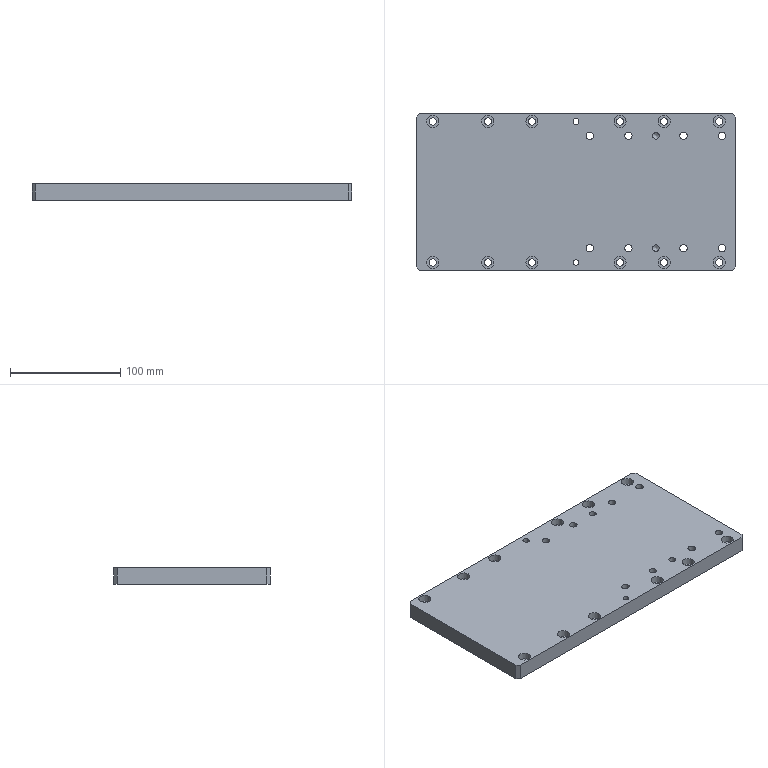Part | 1 solid | 63 faces | box 290 x 142 x 15 mm | volume 601149 mm3 | cylinder 37 | plane 24 | cone 2 | commonest cylinder face diameters 6.6 x12 11 x12 6.8 x8 5 x3 6 x2